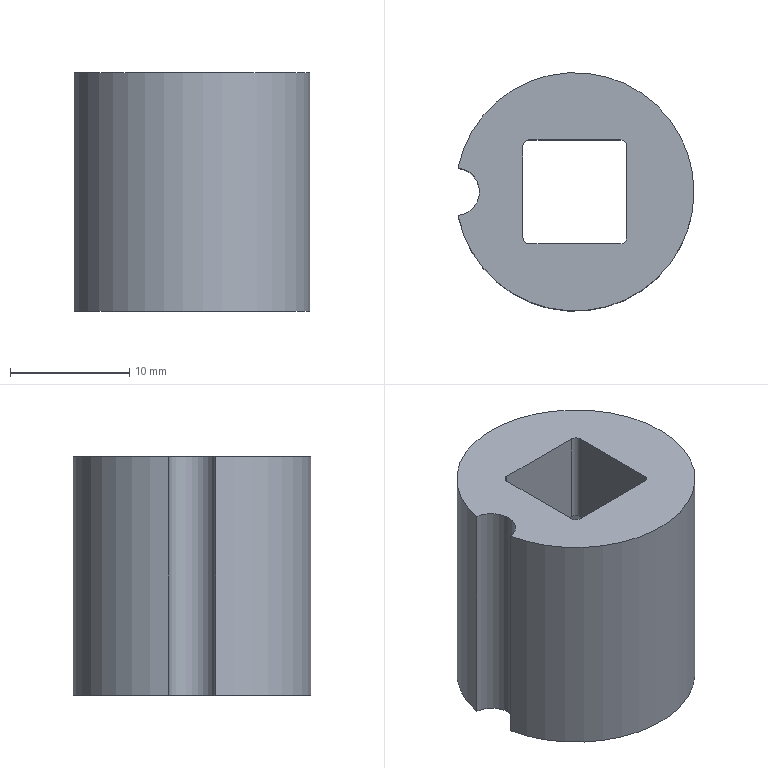Part | NX | features solid 2 | 1 solid | 14 faces | box 19.8 x 20 x 20 mm | volume 4063 mm3 | cylinder 7 | plane 7 | commonest cylinder face diameters 1 x4 4 x1 12.6 x1 20 x1
STEP:
#1=CARTESIAN_POINT('',(331.2,-108.336,-48.));
#2=VERTEX_POINT('',#1);
#3=CARTESIAN_POINT('',(331.2,-108.336,-28.));
#4=VERTEX_POINT('',#3);
#5=CARTESIAN_POINT('',(331.2,-108.336,-38.));
#6=DIRECTION('',(0.,0.,1.));
#7=VECTOR('',#6,1000.);
#8=LINE('',#5,#7);
#9=EDGE_CURVE('',#2,#4,#8,.T.);
#10=ORIENTED_EDGE('',*,*,#9,.F.);
#11=CARTESIAN_POINT('',(331.2,-104.356,-48.));
#12=VERTEX_POINT('',#11);
#13=CARTESIAN_POINT('',(341.,-106.346,-48.));
#14=DIRECTION('',(0.,0.,1.));
#15=DIRECTION('',(-1.,0.,0.));
#16=AXIS2_PLACEMENT_3D('',#13,#14,#15);
#17=CIRCLE('',#16,10.);
#18=EDGE_CURVE('',#2,#12,#17,.T.);
#19=ORIENTED_EDGE('',*,*,#18,.T.);
#20=CARTESIAN_POINT('',(331.2,-104.356,-28.));
#21=VERTEX_POINT('',#20);
#22=CARTESIAN_POINT('',(331.2,-104.356,-38.));
#23=DIRECTION('',(0.,0.,1.));
#24=VECTOR('',#23,1000.);
#25=LINE('',#22,#24);
#26=EDGE_CURVE('',#21,#12,#25,.F.);
#27=ORIENTED_EDGE('',*,*,#26,.F.);
#28=CARTESIAN_POINT('',(341.,-106.346,-28.));
#29=DIRECTION('',(0.,0.,1.));
#30=DIRECTION('',(-1.,0.,0.));
#31=AXIS2_PLACEMENT_3D('',#28,#29,#30);
#32=CIRCLE('',#31,10.);
#33=EDGE_CURVE('',#4,#21,#32,.T.);
#34=ORIENTED_EDGE('',*,*,#33,.F.);
#35=EDGE_LOOP('',(#10,#19,#27,#34));
#36=FACE_BOUND('',#35,.T.);
#37=CARTESIAN_POINT('',(341.,-106.346,-48.));
#38=DIRECTION('',(0.,0.,1.));
#39=DIRECTION('',(-1.,0.,0.));
#40=AXIS2_PLACEMENT_3D('',#37,#38,#39);
#41=CYLINDRICAL_SURFACE('',#40,10.);
#42=ADVANCED_FACE('',(#36),#41,.T.);
#43=CARTESIAN_POINT('',(334.7,-106.346,-48.));
#44=VERTEX_POINT('',#43);
#45=CARTESIAN_POINT('',(341.,-106.346,-48.));
#46=DIRECTION('',(0.,0.,1.));
#47=DIRECTION('',(-1.,0.,0.));
#48=AXIS2_PLACEMENT_3D('',#45,#46,#47);
#49=CIRCLE('',#48,6.3);
#50=EDGE_CURVE('',#44,#44,#49,.T.);
#51=ORIENTED_EDGE('',*,*,#50,.T.);
#52=EDGE_LOOP('',(#51));
#53=FACE_BOUND('',#52,.T.);
#54=ORIENTED_EDGE('',*,*,#18,.F.);
#55=CARTESIAN_POINT('',(331.,-106.346,-48.));
#56=DIRECTION('',(0.,0.,1.));
#57=DIRECTION('',(-1.,0.,0.));
#58=AXIS2_PLACEMENT_3D('',#55,#56,#57);
#59=CIRCLE('',#58,2.);
#60=EDGE_CURVE('',#2,#12,#59,.T.);
#61=ORIENTED_EDGE('',*,*,#60,.T.);
#62=EDGE_LOOP('',(#54,#61));
#63=FACE_BOUND('',#62,.T.);
#64=CARTESIAN_POINT('',(341.,-106.346,-48.));
#65=DIRECTION('',(0.,0.,1.));
#66=DIRECTION('',(-1.,0.,0.));
#67=AXIS2_PLACEMENT_3D('',#64,#65,#66);
#68=PLANE('',#67);
#69=ADVANCED_FACE('',(#53,#63),#68,.F.);
#70=CARTESIAN_POINT('',(345.35,-110.196,-28.));
#71=VERTEX_POINT('',#70);
#72=CARTESIAN_POINT('',(345.35,-102.496,-28.));
#73=VERTEX_POINT('',#72);
#74=CARTESIAN_POINT('',(345.35,-110.696,-28.));
#75=DIRECTION('',(0.,1.,0.));
#76=VECTOR('',#75,1000.);
#77=LINE('',#74,#76);
#78=EDGE_CURVE('',#71,#73,#77,.T.);
#79=ORIENTED_EDGE('',*,*,#78,.F.);
#80=CARTESIAN_POINT('',(344.85,-110.696,-28.));
#81=VERTEX_POINT('',#80);
#82=CARTESIAN_POINT('',(344.85,-110.196,-28.));
#83=DIRECTION('',(0.,0.,1.));
#84=DIRECTION('',(-1.,0.,0.));
#85=AXIS2_PLACEMENT_3D('',#82,#83,#84);
#86=CIRCLE('',#85,0.5);
#87=EDGE_CURVE('',#71,#81,#86,.F.);
#88=ORIENTED_EDGE('',*,*,#87,.T.);
#89=CARTESIAN_POINT('',(337.15,-110.696,-28.));
#90=VERTEX_POINT('',#89);
#91=CARTESIAN_POINT('',(336.65,-110.696,-28.));
#92=DIRECTION('',(1.,0.,0.));
#93=VECTOR('',#92,1000.);
#94=LINE('',#91,#93);
#95=EDGE_CURVE('',#90,#81,#94,.T.);
#96=ORIENTED_EDGE('',*,*,#95,.F.);
#97=CARTESIAN_POINT('',(336.65,-110.196,-28.));
#98=VERTEX_POINT('',#97);
#99=CARTESIAN_POINT('',(337.15,-110.196,-28.));
#100=DIRECTION('',(0.,0.,1.));
#101=DIRECTION('',(-1.,0.,0.));
#102=AXIS2_PLACEMENT_3D('',#99,#100,#101);
#103=CIRCLE('',#102,0.5);
#104=EDGE_CURVE('',#90,#98,#103,.F.);
#105=ORIENTED_EDGE('',*,*,#104,.T.);
#106=CARTESIAN_POINT('',(336.65,-102.496,-28.));
#107=VERTEX_POINT('',#106);
#108=CARTESIAN_POINT('',(336.65,-110.696,-28.));
#109=DIRECTION('',(0.,1.,0.));
#110=VECTOR('',#109,1000.);
#111=LINE('',#108,#110);
#112=EDGE_CURVE('',#98,#107,#111,.T.);
#113=ORIENTED_EDGE('',*,*,#112,.T.);
#114=CARTESIAN_POINT('',(337.15,-101.996,-28.));
#115=VERTEX_POINT('',#114);
#116=CARTESIAN_POINT('',(337.15,-102.496,-28.));
#117=DIRECTION('',(0.,0.,1.));
#118=DIRECTION('',(-1.,0.,0.));
#119=AXIS2_PLACEMENT_3D('',#116,#117,#118);
#120=CIRCLE('',#119,0.5);
#121=EDGE_CURVE('',#107,#115,#120,.F.);
#122=ORIENTED_EDGE('',*,*,#121,.T.);
#123=CARTESIAN_POINT('',(344.85,-101.996,-28.));
#124=VERTEX_POINT('',#123);
#125=CARTESIAN_POINT('',(345.35,-101.996,-28.));
#126=DIRECTION('',(-1.,0.,0.));
#127=VECTOR('',#126,1000.);
#128=LINE('',#125,#127);
#129=EDGE_CURVE('',#124,#115,#128,.T.);
#130=ORIENTED_EDGE('',*,*,#129,.F.);
#131=CARTESIAN_POINT('',(344.85,-102.496,-28.));
#132=DIRECTION('',(0.,0.,1.));
#133=DIRECTION('',(-1.,0.,0.));
#134=AXIS2_PLACEMENT_3D('',#131,#132,#133);
#135=CIRCLE('',#134,0.5);
#136=EDGE_CURVE('',#124,#73,#135,.F.);
#137=ORIENTED_EDGE('',*,*,#136,.T.);
#138=EDGE_LOOP('',(#79,#88,#96,#105,#113,#122,#130,#137));
#139=FACE_BOUND('',#138,.T.);
#140=CARTESIAN_POINT('',(331.,-106.346,-28.));
#141=DIRECTION('',(0.,0.,1.));
#142=DIRECTION('',(-1.,0.,0.));
#143=AXIS2_PLACEMENT_3D('',#140,#141,#142);
#144=CIRCLE('',#143,2.);
#145=EDGE_CURVE('',#4,#21,#144,.T.);
#146=ORIENTED_EDGE('',*,*,#145,.F.);
#147=ORIENTED_EDGE('',*,*,#33,.T.);
#148=EDGE_LOOP('',(#146,#147));
#149=FACE_BOUND('',#148,.T.);
#150=CARTESIAN_POINT('',(341.,-106.346,-28.));
#151=DIRECTION('',(0.,0.,1.));
#152=DIRECTION('',(-1.,0.,0.));
#153=AXIS2_PLACEMENT_3D('',#150,#151,#152);
#154=PLANE('',#153);
#155=ADVANCED_FACE('',(#139,#149),#154,.T.);
#156=ORIENTED_EDGE('',*,*,#50,.F.);
#157=EDGE_LOOP('',(#156));
#158=FACE_BOUND('',#157,.T.);
#159=CARTESIAN_POINT('',(334.7,-106.346,-36.));
#160=VERTEX_POINT('',#159);
#161=CARTESIAN_POINT('',(341.,-106.346,-36.));
#162=DIRECTION('',(0.,0.,1.));
#163=DIRECTION('',(-1.,0.,0.));
#164=AXIS2_PLACEMENT_3D('',#161,#162,#163);
#165=CIRCLE('',#164,6.3);
#166=EDGE_CURVE('',#160,#160,#165,.T.);
#167=ORIENTED_EDGE('',*,*,#166,.T.);
#168=EDGE_LOOP('',(#167));
#169=FACE_BOUND('',#168,.T.);
#170=CARTESIAN_POINT('',(341.,-106.346,-48.));
#171=DIRECTION('',(0.,0.,1.));
#172=DIRECTION('',(-1.,0.,0.));
#173=AXIS2_PLACEMENT_3D('',#170,#171,#172);
#174=CYLINDRICAL_SURFACE('',#173,6.3);
#175=ADVANCED_FACE('',(#158,#169),#174,.F.);
#176=CARTESIAN_POINT('',(336.65,-110.196,-36.));
#177=VERTEX_POINT('',#176);
#178=CARTESIAN_POINT('',(336.65,-102.496,-36.));
#179=VERTEX_POINT('',#178);
#180=CARTESIAN_POINT('',(336.65,-106.346,-36.));
#181=DIRECTION('',(0.,1.,0.));
#182=VECTOR('',#181,1000.);
#183=LINE('',#180,#182);
#184=EDGE_CURVE('',#177,#179,#183,.T.);
#185=ORIENTED_EDGE('',*,*,#184,.F.);
#186=CARTESIAN_POINT('',(337.15,-110.696,-36.));
#187=VERTEX_POINT('',#186);
#188=CARTESIAN_POINT('',(337.15,-110.196,-36.));
#189=DIRECTION('',(0.,0.,1.));
#190=DIRECTION('',(-1.,0.,0.));
#191=AXIS2_PLACEMENT_3D('',#188,#189,#190);
#192=CIRCLE('',#191,0.5);
#193=EDGE_CURVE('',#177,#187,#192,.T.);
#194=ORIENTED_EDGE('',*,*,#193,.T.);
#195=CARTESIAN_POINT('',(344.85,-110.696,-36.));
#196=VERTEX_POINT('',#195);
#197=CARTESIAN_POINT('',(341.,-110.696,-36.));
#198=DIRECTION('',(1.,0.,0.));
#199=VECTOR('',#198,1000.);
#200=LINE('',#197,#199);
#201=EDGE_CURVE('',#187,#196,#200,.T.);
#202=ORIENTED_EDGE('',*,*,#201,.T.);
#203=CARTESIAN_POINT('',(345.35,-110.196,-36.));
#204=VERTEX_POINT('',#203);
#205=CARTESIAN_POINT('',(344.85,-110.196,-36.));
#206=DIRECTION('',(0.,0.,1.));
#207=DIRECTION('',(-1.,0.,0.));
#208=AXIS2_PLACEMENT_3D('',#205,#206,#207);
#209=CIRCLE('',#208,0.5);
#210=EDGE_CURVE('',#196,#204,#209,.T.);
#211=ORIENTED_EDGE('',*,*,#210,.T.);
#212=CARTESIAN_POINT('',(345.35,-102.496,-36.));
#213=VERTEX_POINT('',#212);
#214=CARTESIAN_POINT('',(345.35,-106.346,-36.));
#215=DIRECTION('',(0.,1.,0.));
#216=VECTOR('',#215,1000.);
#217=LINE('',#214,#216);
#218=EDGE_CURVE('',#204,#213,#217,.T.);
#219=ORIENTED_EDGE('',*,*,#218,.T.);
#220=CARTESIAN_POINT('',(344.85,-101.996,-36.));
#221=VERTEX_POINT('',#220);
#222=CARTESIAN_POINT('',(344.85,-102.496,-36.));
#223=DIRECTION('',(0.,0.,1.));
#224=DIRECTION('',(-1.,0.,0.));
#225=AXIS2_PLACEMENT_3D('',#222,#223,#224);
#226=CIRCLE('',#225,0.5);
#227=EDGE_CURVE('',#213,#221,#226,.T.);
#228=ORIENTED_EDGE('',*,*,#227,.T.);
#229=CARTESIAN_POINT('',(337.15,-101.996,-36.));
#230=VERTEX_POINT('',#229);
#231=CARTESIAN_POINT('',(341.,-101.996,-36.));
#232=DIRECTION('',(-1.,0.,0.));
#233=VECTOR('',#232,1000.);
#234=LINE('',#231,#233);
#235=EDGE_CURVE('',#221,#230,#234,.T.);
#236=ORIENTED_EDGE('',*,*,#235,.T.);
#237=CARTESIAN_POINT('',(337.15,-102.496,-36.));
#238=DIRECTION('',(0.,0.,1.));
#239=DIRECTION('',(-1.,0.,0.));
#240=AXIS2_PLACEMENT_3D('',#237,#238,#239);
#241=CIRCLE('',#240,0.5);
#242=EDGE_CURVE('',#230,#179,#241,.T.);
#243=ORIENTED_EDGE('',*,*,#242,.T.);
#244=EDGE_LOOP('',(#185,#194,#202,#211,#219,#228,#236,#243));
#245=FACE_BOUND('',#244,.T.);
#246=ORIENTED_EDGE('',*,*,#166,.F.);
#247=EDGE_LOOP('',(#246));
#248=FACE_BOUND('',#247,.T.);
#249=CARTESIAN_POINT('',(341.,-106.346,-36.));
#250=DIRECTION('',(0.,0.,1.));
#251=DIRECTION('',(-1.,0.,0.));
#252=AXIS2_PLACEMENT_3D('',#249,#250,#251);
#253=PLANE('',#252);
#254=ADVANCED_FACE('',(#245,#248),#253,.F.);
#255=ORIENTED_EDGE('',*,*,#9,.T.);
#256=ORIENTED_EDGE('',*,*,#145,.T.);
#257=ORIENTED_EDGE('',*,*,#26,.T.);
#258=ORIENTED_EDGE('',*,*,#60,.F.);
#259=EDGE_LOOP('',(#255,#256,#257,#258));
#260=FACE_BOUND('',#259,.T.);
#261=CARTESIAN_POINT('',(331.,-106.346,-48.));
#262=DIRECTION('',(0.,0.,1.));
#263=DIRECTION('',(-1.,0.,0.));
#264=AXIS2_PLACEMENT_3D('',#261,#262,#263);
#265=CYLINDRICAL_SURFACE('',#264,2.);
#266=ADVANCED_FACE('',(#260),#265,.F.);
#267=ORIENTED_EDGE('',*,*,#78,.T.);
#268=CARTESIAN_POINT('',(345.35,-102.496,-48.));
#269=DIRECTION('',(0.,0.,-1.));
#270=VECTOR('',#269,1000.);
#271=LINE('',#268,#270);
#272=EDGE_CURVE('',#73,#213,#271,.T.);
#273=ORIENTED_EDGE('',*,*,#272,.T.);
#274=ORIENTED_EDGE('',*,*,#218,.F.);
#275=CARTESIAN_POINT('',(345.35,-110.196,-48.));
#276=DIRECTION('',(0.,0.,-1.));
#277=VECTOR('',#276,1000.);
#278=LINE('',#275,#277);
#279=EDGE_CURVE('',#204,#71,#278,.F.);
#280=ORIENTED_EDGE('',*,*,#279,.T.);
#281=EDGE_LOOP('',(#267,#273,#274,#280));
#282=FACE_BOUND('',#281,.T.);
#283=CARTESIAN_POINT('',(345.35,-110.696,-48.));
#284=DIRECTION('',(1.,0.,0.));
#285=DIRECTION('',(0.,0.,1.));
#286=AXIS2_PLACEMENT_3D('',#283,#284,#285);
#287=PLANE('',#286);
#288=ADVANCED_FACE('',(#282),#287,.F.);
#289=ORIENTED_EDGE('',*,*,#129,.T.);
#290=CARTESIAN_POINT('',(337.15,-101.996,-48.));
#291=DIRECTION('',(0.,0.,-1.));
#292=VECTOR('',#291,1000.);
#293=LINE('',#290,#292);
#294=EDGE_CURVE('',#115,#230,#293,.T.);
#295=ORIENTED_EDGE('',*,*,#294,.T.);
#296=ORIENTED_EDGE('',*,*,#235,.F.);
#297=CARTESIAN_POINT('',(344.85,-101.996,-48.));
#298=DIRECTION('',(0.,0.,-1.));
#299=VECTOR('',#298,1000.);
#300=LINE('',#297,#299);
#301=EDGE_CURVE('',#221,#124,#300,.F.);
#302=ORIENTED_EDGE('',*,*,#301,.T.);
#303=EDGE_LOOP('',(#289,#295,#296,#302));
#304=FACE_BOUND('',#303,.T.);
#305=CARTESIAN_POINT('',(345.35,-101.996,-48.));
#306=DIRECTION('',(0.,1.,0.));
#307=DIRECTION('',(0.,0.,-1.));
#308=AXIS2_PLACEMENT_3D('',#305,#306,#307);
#309=PLANE('',#308);
#310=ADVANCED_FACE('',(#304),#309,.F.);
#311=ORIENTED_EDGE('',*,*,#112,.F.);
#312=CARTESIAN_POINT('',(336.65,-110.196,-48.));
#313=DIRECTION('',(0.,0.,-1.));
#314=VECTOR('',#313,1000.);
#315=LINE('',#312,#314);
#316=EDGE_CURVE('',#98,#177,#315,.T.);
#317=ORIENTED_EDGE('',*,*,#316,.T.);
#318=ORIENTED_EDGE('',*,*,#184,.T.);
#319=CARTESIAN_POINT('',(336.65,-102.496,-48.));
#320=DIRECTION('',(0.,0.,-1.));
#321=VECTOR('',#320,1000.);
#322=LINE('',#319,#321);
#323=EDGE_CURVE('',#179,#107,#322,.F.);
#324=ORIENTED_EDGE('',*,*,#323,.T.);
#325=EDGE_LOOP('',(#311,#317,#318,#324));
#326=FACE_BOUND('',#325,.T.);
#327=CARTESIAN_POINT('',(336.65,-110.696,-48.));
#328=DIRECTION('',(1.,0.,0.));
#329=DIRECTION('',(0.,0.,1.));
#330=AXIS2_PLACEMENT_3D('',#327,#328,#329);
#331=PLANE('',#330);
#332=ADVANCED_FACE('',(#326),#331,.T.);
#333=ORIENTED_EDGE('',*,*,#201,.F.);
#334=CARTESIAN_POINT('',(337.15,-110.696,-48.));
#335=DIRECTION('',(0.,0.,-1.));
#336=VECTOR('',#335,1000.);
#337=LINE('',#334,#336);
#338=EDGE_CURVE('',#187,#90,#337,.F.);
#339=ORIENTED_EDGE('',*,*,#338,.T.);
#340=ORIENTED_EDGE('',*,*,#95,.T.);
#341=CARTESIAN_POINT('',(344.85,-110.696,-48.));
#342=DIRECTION('',(0.,0.,-1.));
#343=VECTOR('',#342,1000.);
#344=LINE('',#341,#343);
#345=EDGE_CURVE('',#81,#196,#344,.T.);
#346=ORIENTED_EDGE('',*,*,#345,.T.);
#347=EDGE_LOOP('',(#333,#339,#340,#346));
#348=FACE_BOUND('',#347,.T.);
#349=CARTESIAN_POINT('',(336.65,-110.696,-48.));
#350=DIRECTION('',(0.,-1.,0.));
#351=DIRECTION('',(0.,0.,1.));
#352=AXIS2_PLACEMENT_3D('',#349,#350,#351);
#353=PLANE('',#352);
#354=ADVANCED_FACE('',(#348),#353,.F.);
#355=ORIENTED_EDGE('',*,*,#193,.F.);
#356=ORIENTED_EDGE('',*,*,#316,.F.);
#357=ORIENTED_EDGE('',*,*,#104,.F.);
#358=ORIENTED_EDGE('',*,*,#338,.F.);
#359=EDGE_LOOP('',(#355,#356,#357,#358));
#360=FACE_BOUND('',#359,.T.);
#361=CARTESIAN_POINT('',(337.15,-110.196,-48.));
#362=DIRECTION('',(0.,0.,-1.));
#363=DIRECTION('',(1.,0.,0.));
#364=AXIS2_PLACEMENT_3D('',#361,#362,#363);
#365=CYLINDRICAL_SURFACE('',#364,0.5);
#366=ADVANCED_FACE('',(#360),#365,.F.);
#367=ORIENTED_EDGE('',*,*,#242,.F.);
#368=ORIENTED_EDGE('',*,*,#294,.F.);
#369=ORIENTED_EDGE('',*,*,#121,.F.);
#370=ORIENTED_EDGE('',*,*,#323,.F.);
#371=EDGE_LOOP('',(#367,#368,#369,#370));
#372=FACE_BOUND('',#371,.T.);
#373=CARTESIAN_POINT('',(337.15,-102.496,-48.));
#374=DIRECTION('',(0.,0.,-1.));
#375=DIRECTION('',(1.,0.,0.));
#376=AXIS2_PLACEMENT_3D('',#373,#374,#375);
#377=CYLINDRICAL_SURFACE('',#376,0.5);
#378=ADVANCED_FACE('',(#372),#377,.F.);
#379=ORIENTED_EDGE('',*,*,#227,.F.);
#380=ORIENTED_EDGE('',*,*,#272,.F.);
#381=ORIENTED_EDGE('',*,*,#136,.F.);
#382=ORIENTED_EDGE('',*,*,#301,.F.);
#383=EDGE_LOOP('',(#379,#380,#381,#382));
#384=FACE_BOUND('',#383,.T.);
#385=CARTESIAN_POINT('',(344.85,-102.496,-48.));
#386=DIRECTION('',(0.,0.,1.));
#387=DIRECTION('',(-1.,0.,0.));
#388=AXIS2_PLACEMENT_3D('',#385,#386,#387);
#389=CYLINDRICAL_SURFACE('',#388,0.5);
#390=ADVANCED_FACE('',(#384),#389,.F.);
#391=ORIENTED_EDGE('',*,*,#210,.F.);
#392=ORIENTED_EDGE('',*,*,#345,.F.);
#393=ORIENTED_EDGE('',*,*,#87,.F.);
#394=ORIENTED_EDGE('',*,*,#279,.F.);
#395=EDGE_LOOP('',(#391,#392,#393,#394));
#396=FACE_BOUND('',#395,.T.);
#397=CARTESIAN_POINT('',(344.85,-110.196,-48.));
#398=DIRECTION('',(0.,0.,1.));
#399=DIRECTION('',(-1.,0.,0.));
#400=AXIS2_PLACEMENT_3D('',#397,#398,#399);
#401=CYLINDRICAL_SURFACE('',#400,0.5);
#402=ADVANCED_FACE('',(#396),#401,.F.);
#403=CLOSED_SHELL('',(#42,#69,#155,#175,#254,#266,#288,#310,#332,#354,#366,#378,#390,#402));
#404=MANIFOLD_SOLID_BREP('',#403);
#405=(LENGTH_UNIT()NAMED_UNIT(*)SI_UNIT(.MILLI.,.METRE.));
#406=UNCERTAINTY_MEASURE_WITH_UNIT(LENGTH_MEASURE(0.00001),#405,'','');
#407=(NAMED_UNIT(*)PLANE_ANGLE_UNIT()SI_UNIT($,.RADIAN.));
#408=(NAMED_UNIT(*)SI_UNIT($,.STERADIAN.)SOLID_ANGLE_UNIT());
#409=(GEOMETRIC_REPRESENTATION_CONTEXT(3)GLOBAL_UNCERTAINTY_ASSIGNED_CONTEXT((#406))GLOBAL_UNIT_ASSIGNED_CONTEXT((#405,#407,#408))REPRESENTATION_CONTEXT('',''));
#410=ADVANCED_BREP_SHAPE_REPRESENTATION('',(#404),#409);